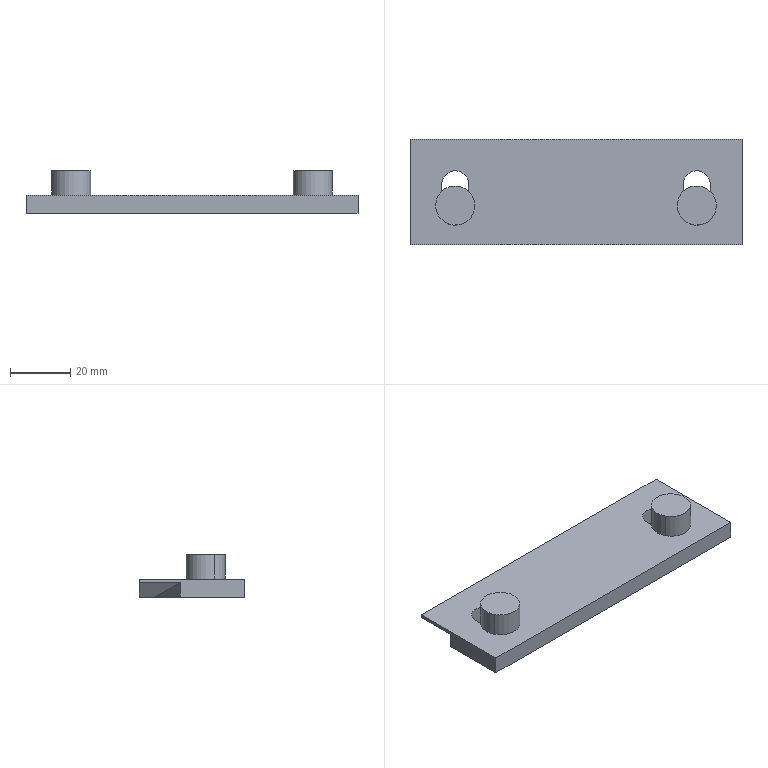Part | CATIA | 3 solids | 26 faces | box 110 x 35 x 14 mm | volume 22917 mm3 | plane 18 | cylinder 8 | commonest cylinder face diameters 9 x4 13 x4
STEP:
#1=CARTESIAN_POINT('',(-55.,-30.,38.));
#2=VERTEX_POINT('',#1);
#3=CARTESIAN_POINT('',(-55.,-30.,44.));
#4=VERTEX_POINT('',#3);
#5=CARTESIAN_POINT('',(-55.,-30.,41.));
#6=DIRECTION('',(0.,0.,1.));
#7=VECTOR('',#6,1.);
#8=LINE('',#5,#7);
#9=EDGE_CURVE('',#2,#4,#8,.T.);
#10=ORIENTED_EDGE('',*,*,#9,.F.);
#11=CARTESIAN_POINT('',(55.,-30.,38.));
#12=VERTEX_POINT('',#11);
#13=CARTESIAN_POINT('',(0.,-30.,38.));
#14=DIRECTION('',(1.,0.,0.));
#15=VECTOR('',#14,1.);
#16=LINE('',#13,#15);
#17=EDGE_CURVE('',#2,#12,#16,.T.);
#18=ORIENTED_EDGE('',*,*,#17,.T.);
#19=CARTESIAN_POINT('',(55.,-30.,44.));
#20=VERTEX_POINT('',#19);
#21=CARTESIAN_POINT('',(55.,-30.,41.));
#22=DIRECTION('',(0.,0.,1.));
#23=VECTOR('',#22,1.);
#24=LINE('',#21,#23);
#25=EDGE_CURVE('',#12,#20,#24,.T.);
#26=ORIENTED_EDGE('',*,*,#25,.T.);
#27=CARTESIAN_POINT('',(0.,-30.,44.));
#28=DIRECTION('',(1.,0.,0.));
#29=VECTOR('',#28,1.);
#30=LINE('',#27,#29);
#31=EDGE_CURVE('',#4,#20,#30,.T.);
#32=ORIENTED_EDGE('',*,*,#31,.F.);
#33=EDGE_LOOP('',(#10,#18,#26,#32));
#34=FACE_OUTER_BOUND('',#33,.T.);
#35=CARTESIAN_POINT('',(-55.,-30.,38.));
#36=DIRECTION('',(0.,-1.,0.));
#37=DIRECTION('',(1.,0.,0.));
#38=AXIS2_PLACEMENT_3D('',#35,#36,#37);
#39=PLANE('',#38);
#40=ADVANCED_FACE('',(#34),#39,.T.);
#41=CARTESIAN_POINT('',(55.,-8.66,42.874));
#42=VERTEX_POINT('',#41);
#43=CARTESIAN_POINT('',(55.,-8.66,38.));
#44=VERTEX_POINT('',#43);
#45=CARTESIAN_POINT('',(55.,-8.66,40.437));
#46=DIRECTION('',(0.,0.,-1.));
#47=VECTOR('',#46,1.);
#48=LINE('',#45,#47);
#49=EDGE_CURVE('',#42,#44,#48,.T.);
#50=ORIENTED_EDGE('',*,*,#49,.F.);
#51=CARTESIAN_POINT('',(55.,5.,42.874));
#52=VERTEX_POINT('',#51);
#53=CARTESIAN_POINT('',(55.,-1.83,42.874));
#54=DIRECTION('',(0.,1.,0.));
#55=VECTOR('',#54,1.);
#56=LINE('',#53,#55);
#57=EDGE_CURVE('',#42,#52,#56,.T.);
#58=ORIENTED_EDGE('',*,*,#57,.T.);
#59=CARTESIAN_POINT('',(55.,5.,44.));
#60=VERTEX_POINT('',#59);
#61=CARTESIAN_POINT('',(55.,5.,43.437));
#62=DIRECTION('',(0.,0.,1.));
#63=VECTOR('',#62,1.);
#64=LINE('',#61,#63);
#65=EDGE_CURVE('',#52,#60,#64,.T.);
#66=ORIENTED_EDGE('',*,*,#65,.T.);
#67=CARTESIAN_POINT('',(55.,-12.5,44.));
#68=DIRECTION('',(0.,-1.,0.));
#69=VECTOR('',#68,1.);
#70=LINE('',#67,#69);
#71=EDGE_CURVE('',#20,#60,#70,.F.);
#72=ORIENTED_EDGE('',*,*,#71,.F.);
#73=ORIENTED_EDGE('',*,*,#25,.F.);
#74=CARTESIAN_POINT('',(55.,-19.33,38.));
#75=DIRECTION('',(0.,-1.,0.));
#76=VECTOR('',#75,1.);
#77=LINE('',#74,#76);
#78=EDGE_CURVE('',#12,#44,#77,.F.);
#79=ORIENTED_EDGE('',*,*,#78,.T.);
#80=EDGE_LOOP('',(#50,#58,#66,#72,#73,#79));
#81=FACE_OUTER_BOUND('',#80,.T.);
#82=CARTESIAN_POINT('',(55.,5.,38.));
#83=DIRECTION('',(-1.,0.,0.));
#84=DIRECTION('',(0.,-1.,0.));
#85=AXIS2_PLACEMENT_3D('',#82,#83,#84);
#86=PLANE('',#85);
#87=ADVANCED_FACE('',(#81),#86,.F.);
#88=CARTESIAN_POINT('',(-55.,-8.66,42.874));
#89=VERTEX_POINT('',#88);
#90=CARTESIAN_POINT('',(-55.,5.,42.874));
#91=VERTEX_POINT('',#90);
#92=CARTESIAN_POINT('',(-55.,-1.83,42.874));
#93=DIRECTION('',(0.,1.,0.));
#94=VECTOR('',#93,1.);
#95=LINE('',#92,#94);
#96=EDGE_CURVE('',#89,#91,#95,.T.);
#97=ORIENTED_EDGE('',*,*,#96,.F.);
#98=CARTESIAN_POINT('',(-55.,-8.66,38.));
#99=VERTEX_POINT('',#98);
#100=CARTESIAN_POINT('',(-55.,-8.66,40.437));
#101=DIRECTION('',(0.,0.,-1.));
#102=VECTOR('',#101,1.);
#103=LINE('',#100,#102);
#104=EDGE_CURVE('',#89,#99,#103,.T.);
#105=ORIENTED_EDGE('',*,*,#104,.T.);
#106=CARTESIAN_POINT('',(-55.,-19.33,38.));
#107=DIRECTION('',(0.,1.,0.));
#108=VECTOR('',#107,1.);
#109=LINE('',#106,#108);
#110=EDGE_CURVE('',#99,#2,#109,.F.);
#111=ORIENTED_EDGE('',*,*,#110,.T.);
#112=ORIENTED_EDGE('',*,*,#9,.T.);
#113=CARTESIAN_POINT('',(-55.,5.,44.));
#114=VERTEX_POINT('',#113);
#115=CARTESIAN_POINT('',(-55.,-12.5,44.));
#116=DIRECTION('',(0.,1.,0.));
#117=VECTOR('',#116,1.);
#118=LINE('',#115,#117);
#119=EDGE_CURVE('',#114,#4,#118,.F.);
#120=ORIENTED_EDGE('',*,*,#119,.F.);
#121=CARTESIAN_POINT('',(-55.,5.,43.437));
#122=DIRECTION('',(0.,0.,1.));
#123=VECTOR('',#122,1.);
#124=LINE('',#121,#123);
#125=EDGE_CURVE('',#91,#114,#124,.T.);
#126=ORIENTED_EDGE('',*,*,#125,.F.);
#127=EDGE_LOOP('',(#97,#105,#111,#112,#120,#126));
#128=FACE_OUTER_BOUND('',#127,.T.);
#129=CARTESIAN_POINT('',(-55.,-30.,38.));
#130=DIRECTION('',(1.,0.,0.));
#131=DIRECTION('',(0.,1.,0.));
#132=AXIS2_PLACEMENT_3D('',#129,#130,#131);
#133=PLANE('',#132);
#134=ADVANCED_FACE('',(#128),#133,.F.);
#135=CARTESIAN_POINT('',(40.,5.,38.));
#136=VERTEX_POINT('',#135);
#137=CARTESIAN_POINT('',(-40.,5.,38.));
#138=VERTEX_POINT('',#137);
#139=CARTESIAN_POINT('',(0.,5.,38.));
#140=DIRECTION('',(-1.,0.,0.));
#141=VECTOR('',#140,1.);
#142=LINE('',#139,#141);
#143=EDGE_CURVE('',#136,#138,#142,.T.);
#144=ORIENTED_EDGE('',*,*,#143,.T.);
#145=CARTESIAN_POINT('',(-47.5,5.,40.437));
#146=DIRECTION('',(-0.9511,0.,0.309));
#147=VECTOR('',#146,1.);
#148=LINE('',#145,#147);
#149=EDGE_CURVE('',#138,#91,#148,.T.);
#150=ORIENTED_EDGE('',*,*,#149,.T.);
#151=ORIENTED_EDGE('',*,*,#125,.T.);
#152=CARTESIAN_POINT('',(0.,5.,44.));
#153=DIRECTION('',(-1.,0.,0.));
#154=VECTOR('',#153,1.);
#155=LINE('',#152,#154);
#156=EDGE_CURVE('',#60,#114,#155,.T.);
#157=ORIENTED_EDGE('',*,*,#156,.F.);
#158=ORIENTED_EDGE('',*,*,#65,.F.);
#159=CARTESIAN_POINT('',(47.5,5.,40.437));
#160=DIRECTION('',(0.9511,0.,0.309));
#161=VECTOR('',#160,1.);
#162=LINE('',#159,#161);
#163=EDGE_CURVE('',#136,#52,#162,.T.);
#164=ORIENTED_EDGE('',*,*,#163,.F.);
#165=EDGE_LOOP('',(#144,#150,#151,#157,#158,#164));
#166=FACE_OUTER_BOUND('',#165,.T.);
#167=CARTESIAN_POINT('',(55.,5.,38.));
#168=DIRECTION('',(0.,1.,0.));
#169=DIRECTION('',(-1.,0.,0.));
#170=AXIS2_PLACEMENT_3D('',#167,#168,#169);
#171=PLANE('',#170);
#172=ADVANCED_FACE('',(#166),#171,.T.);
#173=CARTESIAN_POINT('',(40.,0.,38.));
#174=VERTEX_POINT('',#173);
#175=CARTESIAN_POINT('',(55.,-8.66,42.874));
#176=CARTESIAN_POINT('',(40.,0.,38.));
#177=B_SPLINE_CURVE_WITH_KNOTS('',1,(#175,#176),.UNSPECIFIED.,.F.,.U.,(2,2),(-2.999,14.994),.UNSPECIFIED.);
#178=EDGE_CURVE('',#174,#42,#177,.F.);
#179=ORIENTED_EDGE('',*,*,#178,.T.);
#180=ORIENTED_EDGE('',*,*,#49,.T.);
#181=CARTESIAN_POINT('',(52.5,-7.217,38.));
#182=DIRECTION('',(0.866,-0.5,0.));
#183=VECTOR('',#182,1.);
#184=LINE('',#181,#183);
#185=EDGE_CURVE('',#174,#44,#184,.T.);
#186=ORIENTED_EDGE('',*,*,#185,.F.);
#187=EDGE_LOOP('',(#179,#180,#186));
#188=FACE_OUTER_BOUND('',#187,.T.);
#189=CARTESIAN_POINT('',(40.,0.,38.));
#190=DIRECTION('',(0.5,0.866,0.));
#191=DIRECTION('',(0.,0.,1.));
#192=AXIS2_PLACEMENT_3D('',#189,#190,#191);
#193=PLANE('',#192);
#194=ADVANCED_FACE('',(#188),#193,.T.);
#195=ORIENTED_EDGE('',*,*,#163,.T.);
#196=ORIENTED_EDGE('',*,*,#57,.F.);
#197=ORIENTED_EDGE('',*,*,#178,.F.);
#198=CARTESIAN_POINT('',(40.,5.,38.));
#199=DIRECTION('',(0.,-1.,0.));
#200=VECTOR('',#199,1.);
#201=LINE('',#198,#200);
#202=EDGE_CURVE('',#174,#136,#201,.F.);
#203=ORIENTED_EDGE('',*,*,#202,.T.);
#204=EDGE_LOOP('',(#195,#196,#197,#203));
#205=FACE_OUTER_BOUND('',#204,.T.);
#206=CARTESIAN_POINT('',(40.,10.,38.));
#207=DIRECTION('',(-0.309,0.,0.9511));
#208=DIRECTION('',(0.,-1.,0.));
#209=AXIS2_PLACEMENT_3D('',#206,#207,#208);
#210=PLANE('',#209);
#211=ADVANCED_FACE('',(#205),#210,.F.);
#212=CARTESIAN_POINT('',(-40.,0.,38.));
#213=VERTEX_POINT('',#212);
#214=CARTESIAN_POINT('',(-52.5,-7.217,38.));
#215=DIRECTION('',(-0.866,-0.5,0.));
#216=VECTOR('',#215,1.);
#217=LINE('',#214,#216);
#218=EDGE_CURVE('',#213,#99,#217,.T.);
#219=ORIENTED_EDGE('',*,*,#218,.T.);
#220=ORIENTED_EDGE('',*,*,#104,.F.);
#221=CARTESIAN_POINT('',(-55.,-8.66,42.874));
#222=CARTESIAN_POINT('',(-40.,0.,38.));
#223=B_SPLINE_CURVE_WITH_KNOTS('',1,(#221,#222),.UNSPECIFIED.,.F.,.U.,(2,2),(-2.999,14.994),.UNSPECIFIED.);
#224=EDGE_CURVE('',#213,#89,#223,.F.);
#225=ORIENTED_EDGE('',*,*,#224,.F.);
#226=EDGE_LOOP('',(#219,#220,#225));
#227=FACE_OUTER_BOUND('',#226,.T.);
#228=CARTESIAN_POINT('',(-40.,0.,38.));
#229=DIRECTION('',(0.5,-0.866,0.));
#230=DIRECTION('',(0.,0.,1.));
#231=AXIS2_PLACEMENT_3D('',#228,#229,#230);
#232=PLANE('',#231);
#233=ADVANCED_FACE('',(#227),#232,.F.);
#234=CARTESIAN_POINT('',(-40.,5.,38.));
#235=DIRECTION('',(0.,-1.,0.));
#236=VECTOR('',#235,1.);
#237=LINE('',#234,#236);
#238=EDGE_CURVE('',#213,#138,#237,.F.);
#239=ORIENTED_EDGE('',*,*,#238,.F.);
#240=ORIENTED_EDGE('',*,*,#224,.T.);
#241=ORIENTED_EDGE('',*,*,#96,.T.);
#242=ORIENTED_EDGE('',*,*,#149,.F.);
#243=EDGE_LOOP('',(#239,#240,#241,#242));
#244=FACE_OUTER_BOUND('',#243,.T.);
#245=CARTESIAN_POINT('',(-40.,10.,38.));
#246=DIRECTION('',(-0.309,0.,-0.9511));
#247=DIRECTION('',(0.,-1.,0.));
#248=AXIS2_PLACEMENT_3D('',#245,#246,#247);
#249=PLANE('',#248);
#250=ADVANCED_FACE('',(#244),#249,.T.);
#251=ORIENTED_EDGE('',*,*,#143,.F.);
#252=ORIENTED_EDGE('',*,*,#202,.F.);
#253=ORIENTED_EDGE('',*,*,#185,.T.);
#254=ORIENTED_EDGE('',*,*,#78,.F.);
#255=ORIENTED_EDGE('',*,*,#17,.F.);
#256=ORIENTED_EDGE('',*,*,#110,.F.);
#257=ORIENTED_EDGE('',*,*,#218,.F.);
#258=ORIENTED_EDGE('',*,*,#238,.T.);
#259=EDGE_LOOP('',(#251,#252,#253,#254,#255,#256,#257,#258));
#260=FACE_OUTER_BOUND('',#259,.T.);
#261=CARTESIAN_POINT('',(-35.5,-10.,38.));
#262=VERTEX_POINT('',#261);
#263=CARTESIAN_POINT('',(-35.5,-17.,38.));
#264=VERTEX_POINT('',#263);
#265=CARTESIAN_POINT('',(-35.5,-13.5,38.));
#266=DIRECTION('',(0.,-1.,0.));
#267=VECTOR('',#266,1.);
#268=LINE('',#265,#267);
#269=EDGE_CURVE('',#262,#264,#268,.T.);
#270=ORIENTED_EDGE('',*,*,#269,.F.);
#271=CARTESIAN_POINT('',(-44.5,-10.,38.));
#272=VERTEX_POINT('',#271);
#273=CARTESIAN_POINT('',(-40.,-10.,38.));
#274=DIRECTION('',(0.,0.,1.));
#275=AXIS2_PLACEMENT_3D('',#273,#274,$);
#276=CIRCLE('',#275,4.5);
#277=EDGE_CURVE('',#262,#272,#276,.T.);
#278=ORIENTED_EDGE('',*,*,#277,.T.);
#279=CARTESIAN_POINT('',(-44.5,-17.,38.));
#280=VERTEX_POINT('',#279);
#281=CARTESIAN_POINT('',(-44.5,-13.5,38.));
#282=DIRECTION('',(0.,-1.,0.));
#283=VECTOR('',#282,1.);
#284=LINE('',#281,#283);
#285=EDGE_CURVE('',#272,#280,#284,.T.);
#286=ORIENTED_EDGE('',*,*,#285,.T.);
#287=CARTESIAN_POINT('',(-40.,-17.,38.));
#288=DIRECTION('',(0.,0.,1.));
#289=AXIS2_PLACEMENT_3D('',#287,#288,$);
#290=CIRCLE('',#289,4.5);
#291=EDGE_CURVE('',#280,#264,#290,.T.);
#292=ORIENTED_EDGE('',*,*,#291,.T.);
#293=EDGE_LOOP('',(#270,#278,#286,#292));
#294=FACE_BOUND('',#293,.T.);
#295=CARTESIAN_POINT('',(44.5,-10.,38.));
#296=VERTEX_POINT('',#295);
#297=CARTESIAN_POINT('',(35.5,-10.,38.));
#298=VERTEX_POINT('',#297);
#299=CARTESIAN_POINT('',(40.,-10.,38.));
#300=DIRECTION('',(0.,0.,1.));
#301=AXIS2_PLACEMENT_3D('',#299,#300,$);
#302=CIRCLE('',#301,4.5);
#303=EDGE_CURVE('',#296,#298,#302,.T.);
#304=ORIENTED_EDGE('',*,*,#303,.T.);
#305=CARTESIAN_POINT('',(35.5,-17.,38.));
#306=VERTEX_POINT('',#305);
#307=CARTESIAN_POINT('',(35.5,-13.5,38.));
#308=DIRECTION('',(0.,-1.,0.));
#309=VECTOR('',#308,1.);
#310=LINE('',#307,#309);
#311=EDGE_CURVE('',#298,#306,#310,.T.);
#312=ORIENTED_EDGE('',*,*,#311,.T.);
#313=CARTESIAN_POINT('',(44.5,-17.,38.));
#314=VERTEX_POINT('',#313);
#315=CARTESIAN_POINT('',(40.,-17.,38.));
#316=DIRECTION('',(0.,0.,1.));
#317=AXIS2_PLACEMENT_3D('',#315,#316,$);
#318=CIRCLE('',#317,4.5);
#319=EDGE_CURVE('',#306,#314,#318,.T.);
#320=ORIENTED_EDGE('',*,*,#319,.T.);
#321=CARTESIAN_POINT('',(44.5,-13.5,38.));
#322=DIRECTION('',(0.,-1.,0.));
#323=VECTOR('',#322,1.);
#324=LINE('',#321,#323);
#325=EDGE_CURVE('',#296,#314,#324,.T.);
#326=ORIENTED_EDGE('',*,*,#325,.F.);
#327=EDGE_LOOP('',(#304,#312,#320,#326));
#328=FACE_BOUND('',#327,.T.);
#329=CARTESIAN_POINT('',(0.,0.,38.));
#330=DIRECTION('',(0.,0.,1.));
#331=DIRECTION('',(1.,0.,0.));
#332=AXIS2_PLACEMENT_3D('',#329,#330,#331);
#333=PLANE('',#332);
#334=ADVANCED_FACE('',(#260,#294,#328),#333,.F.);
#335=ORIENTED_EDGE('',*,*,#156,.T.);
#336=ORIENTED_EDGE('',*,*,#119,.T.);
#337=ORIENTED_EDGE('',*,*,#31,.T.);
#338=ORIENTED_EDGE('',*,*,#71,.T.);
#339=EDGE_LOOP('',(#335,#336,#337,#338));
#340=FACE_OUTER_BOUND('',#339,.T.);
#341=CARTESIAN_POINT('',(-35.5,-17.,44.));
#342=VERTEX_POINT('',#341);
#343=CARTESIAN_POINT('',(-35.5,-10.,44.));
#344=VERTEX_POINT('',#343);
#345=CARTESIAN_POINT('',(-35.5,-13.5,44.));
#346=DIRECTION('',(0.,-1.,0.));
#347=VECTOR('',#346,1.);
#348=LINE('',#345,#347);
#349=EDGE_CURVE('',#342,#344,#348,.F.);
#350=ORIENTED_EDGE('',*,*,#349,.F.);
#351=CARTESIAN_POINT('',(-44.5,-17.,44.));
#352=VERTEX_POINT('',#351);
#353=CARTESIAN_POINT('',(-40.,-17.,44.));
#354=DIRECTION('',(0.,0.,1.));
#355=AXIS2_PLACEMENT_3D('',#353,#354,$);
#356=CIRCLE('',#355,4.5);
#357=EDGE_CURVE('',#352,#342,#356,.T.);
#358=ORIENTED_EDGE('',*,*,#357,.F.);
#359=CARTESIAN_POINT('',(-44.5,-10.,44.));
#360=VERTEX_POINT('',#359);
#361=CARTESIAN_POINT('',(-44.5,-13.5,44.));
#362=DIRECTION('',(0.,-1.,0.));
#363=VECTOR('',#362,1.);
#364=LINE('',#361,#363);
#365=EDGE_CURVE('',#360,#352,#364,.T.);
#366=ORIENTED_EDGE('',*,*,#365,.F.);
#367=CARTESIAN_POINT('',(-40.,-10.,44.));
#368=DIRECTION('',(0.,0.,1.));
#369=AXIS2_PLACEMENT_3D('',#367,#368,$);
#370=CIRCLE('',#369,4.5);
#371=EDGE_CURVE('',#344,#360,#370,.T.);
#372=ORIENTED_EDGE('',*,*,#371,.F.);
#373=EDGE_LOOP('',(#350,#358,#366,#372));
#374=FACE_BOUND('',#373,.T.);
#375=CARTESIAN_POINT('',(44.5,-10.,44.));
#376=VERTEX_POINT('',#375);
#377=CARTESIAN_POINT('',(35.5,-10.,44.));
#378=VERTEX_POINT('',#377);
#379=CARTESIAN_POINT('',(40.,-10.,44.));
#380=DIRECTION('',(0.,0.,1.));
#381=AXIS2_PLACEMENT_3D('',#379,#380,$);
#382=CIRCLE('',#381,4.5);
#383=EDGE_CURVE('',#376,#378,#382,.T.);
#384=ORIENTED_EDGE('',*,*,#383,.F.);
#385=CARTESIAN_POINT('',(44.5,-17.,44.));
#386=VERTEX_POINT('',#385);
#387=CARTESIAN_POINT('',(44.5,-13.5,44.));
#388=DIRECTION('',(0.,-1.,0.));
#389=VECTOR('',#388,1.);
#390=LINE('',#387,#389);
#391=EDGE_CURVE('',#386,#376,#390,.F.);
#392=ORIENTED_EDGE('',*,*,#391,.F.);
#393=CARTESIAN_POINT('',(35.5,-17.,44.));
#394=VERTEX_POINT('',#393);
#395=CARTESIAN_POINT('',(40.,-17.,44.));
#396=DIRECTION('',(0.,0.,1.));
#397=AXIS2_PLACEMENT_3D('',#395,#396,$);
#398=CIRCLE('',#397,4.5);
#399=EDGE_CURVE('',#394,#386,#398,.T.);
#400=ORIENTED_EDGE('',*,*,#399,.F.);
#401=CARTESIAN_POINT('',(35.5,-13.5,44.));
#402=DIRECTION('',(0.,-1.,0.));
#403=VECTOR('',#402,1.);
#404=LINE('',#401,#403);
#405=EDGE_CURVE('',#378,#394,#404,.T.);
#406=ORIENTED_EDGE('',*,*,#405,.F.);
#407=EDGE_LOOP('',(#384,#392,#400,#406));
#408=FACE_BOUND('',#407,.T.);
#409=CARTESIAN_POINT('',(0.,0.,44.));
#410=DIRECTION('',(0.,0.,1.));
#411=DIRECTION('',(1.,0.,0.));
#412=AXIS2_PLACEMENT_3D('',#409,#410,#411);
#413=PLANE('',#412);
#414=ADVANCED_FACE('',(#340,#374,#408),#413,.T.);
#415=ORIENTED_EDGE('',*,*,#303,.F.);
#416=CARTESIAN_POINT('',(44.5,-10.,34.));
#417=DIRECTION('',(0.,0.,1.));
#418=VECTOR('',#417,1.);
#419=LINE('',#416,#418);
#420=EDGE_CURVE('',#376,#296,#419,.F.);
#421=ORIENTED_EDGE('',*,*,#420,.F.);
#422=ORIENTED_EDGE('',*,*,#383,.T.);
#423=CARTESIAN_POINT('',(35.5,-10.,34.));
#424=DIRECTION('',(0.,0.,1.));
#425=VECTOR('',#424,1.);
#426=LINE('',#423,#425);
#427=EDGE_CURVE('',#378,#298,#426,.F.);
#428=ORIENTED_EDGE('',*,*,#427,.T.);
#429=EDGE_LOOP('',(#415,#421,#422,#428));
#430=FACE_OUTER_BOUND('',#429,.T.);
#431=CARTESIAN_POINT('',(40.,-10.,34.));
#432=DIRECTION('',(0.,0.,1.));
#433=DIRECTION('',(1.,0.,0.));
#434=AXIS2_PLACEMENT_3D('',#431,#432,#433);
#435=CYLINDRICAL_SURFACE('',#434,4.5);
#436=ADVANCED_FACE('',(#430),#435,.F.);
#437=ORIENTED_EDGE('',*,*,#427,.F.);
#438=ORIENTED_EDGE('',*,*,#405,.T.);
#439=CARTESIAN_POINT('',(35.5,-17.,41.));
#440=DIRECTION('',(0.,0.,-1.));
#441=VECTOR('',#440,1.);
#442=LINE('',#439,#441);
#443=EDGE_CURVE('',#394,#306,#442,.T.);
#444=ORIENTED_EDGE('',*,*,#443,.T.);
#445=ORIENTED_EDGE('',*,*,#311,.F.);
#446=EDGE_LOOP('',(#437,#438,#444,#445));
#447=FACE_OUTER_BOUND('',#446,.T.);
#448=CARTESIAN_POINT('',(35.5,-10.,44.));
#449=DIRECTION('',(1.,0.,0.));
#450=DIRECTION('',(0.,-1.,0.));
#451=AXIS2_PLACEMENT_3D('',#448,#449,#450);
#452=PLANE('',#451);
#453=ADVANCED_FACE('',(#447),#452,.T.);
#454=ORIENTED_EDGE('',*,*,#325,.T.);
#455=CARTESIAN_POINT('',(44.5,-17.,41.));
#456=DIRECTION('',(0.,0.,-1.));
#457=VECTOR('',#456,1.);
#458=LINE('',#455,#457);
#459=EDGE_CURVE('',#386,#314,#458,.T.);
#460=ORIENTED_EDGE('',*,*,#459,.F.);
#461=ORIENTED_EDGE('',*,*,#391,.T.);
#462=ORIENTED_EDGE('',*,*,#420,.T.);
#463=EDGE_LOOP('',(#454,#460,#461,#462));
#464=FACE_OUTER_BOUND('',#463,.T.);
#465=CARTESIAN_POINT('',(44.5,-10.,44.));
#466=DIRECTION('',(1.,0.,0.));
#467=DIRECTION('',(0.,-1.,0.));
#468=AXIS2_PLACEMENT_3D('',#465,#466,#467);
#469=PLANE('',#468);
#470=ADVANCED_FACE('',(#464),#469,.F.);
#471=ORIENTED_EDGE('',*,*,#319,.F.);
#472=ORIENTED_EDGE('',*,*,#443,.F.);
#473=ORIENTED_EDGE('',*,*,#399,.T.);
#474=ORIENTED_EDGE('',*,*,#459,.T.);
#475=EDGE_LOOP('',(#471,#472,#473,#474));
#476=FACE_OUTER_BOUND('',#475,.T.);
#477=CARTESIAN_POINT('',(40.,-17.,34.));
#478=DIRECTION('',(0.,0.,1.));
#479=DIRECTION('',(-1.,0.,0.));
#480=AXIS2_PLACEMENT_3D('',#477,#478,#479);
#481=CYLINDRICAL_SURFACE('',#480,4.5);
#482=ADVANCED_FACE('',(#476),#481,.F.);
#483=ORIENTED_EDGE('',*,*,#269,.T.);
#484=CARTESIAN_POINT('',(-35.5,-17.,41.));
#485=DIRECTION('',(0.,0.,-1.));
#486=VECTOR('',#485,1.);
#487=LINE('',#484,#486);
#488=EDGE_CURVE('',#342,#264,#487,.T.);
#489=ORIENTED_EDGE('',*,*,#488,.F.);
#490=ORIENTED_EDGE('',*,*,#349,.T.);
#491=CARTESIAN_POINT('',(-35.5,-10.,41.));
#492=DIRECTION('',(0.,0.,-1.));
#493=VECTOR('',#492,1.);
#494=LINE('',#491,#493);
#495=EDGE_CURVE('',#344,#262,#494,.T.);
#496=ORIENTED_EDGE('',*,*,#495,.T.);
#497=EDGE_LOOP('',(#483,#489,#490,#496));
#498=FACE_OUTER_BOUND('',#497,.T.);
#499=CARTESIAN_POINT('',(-35.5,-10.,44.));
#500=DIRECTION('',(1.,0.,0.));
#501=DIRECTION('',(0.,-1.,0.));
#502=AXIS2_PLACEMENT_3D('',#499,#500,#501);
#503=PLANE('',#502);
#504=ADVANCED_FACE('',(#498),#503,.F.);
#505=ORIENTED_EDGE('',*,*,#277,.F.);
#506=ORIENTED_EDGE('',*,*,#495,.F.);
#507=ORIENTED_EDGE('',*,*,#371,.T.);
#508=CARTESIAN_POINT('',(-44.5,-10.,34.));
#509=DIRECTION('',(0.,0.,1.));
#510=VECTOR('',#509,1.);
#511=LINE('',#508,#510);
#512=EDGE_CURVE('',#360,#272,#511,.F.);
#513=ORIENTED_EDGE('',*,*,#512,.T.);
#514=EDGE_LOOP('',(#505,#506,#507,#513));
#515=FACE_OUTER_BOUND('',#514,.T.);
#516=CARTESIAN_POINT('',(-40.,-10.,34.));
#517=DIRECTION('',(0.,0.,1.));
#518=DIRECTION('',(1.,0.,0.));
#519=AXIS2_PLACEMENT_3D('',#516,#517,#518);
#520=CYLINDRICAL_SURFACE('',#519,4.5);
#521=ADVANCED_FACE('',(#515),#520,.F.);
#522=ORIENTED_EDGE('',*,*,#291,.F.);
#523=CARTESIAN_POINT('',(-44.5,-17.,34.));
#524=DIRECTION('',(0.,0.,1.));
#525=VECTOR('',#524,1.);
#526=LINE('',#523,#525);
#527=EDGE_CURVE('',#352,#280,#526,.F.);
#528=ORIENTED_EDGE('',*,*,#527,.F.);
#529=ORIENTED_EDGE('',*,*,#357,.T.);
#530=ORIENTED_EDGE('',*,*,#488,.T.);
#531=EDGE_LOOP('',(#522,#528,#529,#530));
#532=FACE_OUTER_BOUND('',#531,.T.);
#533=CARTESIAN_POINT('',(-40.,-17.,34.));
#534=DIRECTION('',(0.,0.,1.));
#535=DIRECTION('',(-1.,0.,0.));
#536=AXIS2_PLACEMENT_3D('',#533,#534,#535);
#537=CYLINDRICAL_SURFACE('',#536,4.5);
#538=ADVANCED_FACE('',(#532),#537,.F.);
#539=ORIENTED_EDGE('',*,*,#512,.F.);
#540=ORIENTED_EDGE('',*,*,#365,.T.);
#541=ORIENTED_EDGE('',*,*,#527,.T.);
#542=ORIENTED_EDGE('',*,*,#285,.F.);
#543=EDGE_LOOP('',(#539,#540,#541,#542));
#544=FACE_OUTER_BOUND('',#543,.T.);
#545=CARTESIAN_POINT('',(-44.5,-10.,44.));
#546=DIRECTION('',(1.,0.,0.));
#547=DIRECTION('',(0.,-1.,0.));
#548=AXIS2_PLACEMENT_3D('',#545,#546,#547);
#549=PLANE('',#548);
#550=ADVANCED_FACE('',(#544),#549,.T.);
#551=CLOSED_SHELL('',(#40,#87,#134,#172,#194,#211,#233,#250,#334,#414,#436,#453,#470,#482,#504,#521,#538,#550));
#552=MANIFOLD_SOLID_BREP('',#551);
#553=CARTESIAN_POINT('',(-34.296,-13.884,52.));
#554=VERTEX_POINT('',#553);
#555=CARTESIAN_POINT('',(-45.704,-20.116,52.));
#556=VERTEX_POINT('',#555);
#557=CARTESIAN_POINT('',(-40.,-17.,52.));
#558=DIRECTION('',(0.,0.,1.));
#559=AXIS2_PLACEMENT_3D('',#557,#558,$);
#560=CIRCLE('',#559,6.5);
#561=EDGE_CURVE('',#554,#556,#560,.T.);
#562=ORIENTED_EDGE('',*,*,#561,.T.);
#563=CARTESIAN_POINT('',(-40.,-17.,52.));
#564=DIRECTION('',(0.,0.,1.));
#565=AXIS2_PLACEMENT_3D('',#563,#564,$);
#566=CIRCLE('',#565,6.5);
#567=EDGE_CURVE('',#556,#554,#566,.T.);
#568=ORIENTED_EDGE('',*,*,#567,.T.);
#569=EDGE_LOOP('',(#562,#568));
#570=FACE_OUTER_BOUND('',#569,.T.);
#571=CARTESIAN_POINT('',(-40.,-17.,52.));
#572=DIRECTION('',(0.,0.,1.));
#573=DIRECTION('',(1.,0.,0.));
#574=AXIS2_PLACEMENT_3D('',#571,#572,#573);
#575=PLANE('',#574);
#576=ADVANCED_FACE('',(#570),#575,.T.);
#577=CARTESIAN_POINT('',(-45.704,-20.116,44.));
#578=VERTEX_POINT('',#577);
#579=CARTESIAN_POINT('',(-45.704,-20.116,47.8));
#580=DIRECTION('',(0.,0.,1.));
#581=VECTOR('',#580,1.);
#582=LINE('',#579,#581);
#583=EDGE_CURVE('',#556,#578,#582,.F.);
#584=ORIENTED_EDGE('',*,*,#583,.F.);
#585=ORIENTED_EDGE('',*,*,#561,.F.);
#586=CARTESIAN_POINT('',(-34.296,-13.884,44.));
#587=VERTEX_POINT('',#586);
#588=CARTESIAN_POINT('',(-34.296,-13.884,47.8));
#589=DIRECTION('',(0.,0.,1.));
#590=VECTOR('',#589,1.);
#591=LINE('',#588,#590);
#592=EDGE_CURVE('',#554,#587,#591,.F.);
#593=ORIENTED_EDGE('',*,*,#592,.T.);
#594=CARTESIAN_POINT('',(-40.,-17.,44.));
#595=DIRECTION('',(0.,0.,1.));
#596=AXIS2_PLACEMENT_3D('',#594,#595,$);
#597=CIRCLE('',#596,6.5);
#598=EDGE_CURVE('',#587,#578,#597,.T.);
#599=ORIENTED_EDGE('',*,*,#598,.T.);
#600=EDGE_LOOP('',(#584,#585,#593,#599));
#601=FACE_OUTER_BOUND('',#600,.T.);
#602=CARTESIAN_POINT('',(-40.,-17.,44.1));
#603=DIRECTION('',(0.,0.,1.));
#604=DIRECTION('',(0.8776,0.4794,0.));
#605=AXIS2_PLACEMENT_3D('',#602,#603,#604);
#606=CYLINDRICAL_SURFACE('',#605,6.5);
#607=ADVANCED_FACE('',(#601),#606,.T.);
#608=ORIENTED_EDGE('',*,*,#592,.F.);
#609=ORIENTED_EDGE('',*,*,#567,.F.);
#610=ORIENTED_EDGE('',*,*,#583,.T.);
#611=CARTESIAN_POINT('',(-40.,-17.,44.));
#612=DIRECTION('',(0.,0.,1.));
#613=AXIS2_PLACEMENT_3D('',#611,#612,$);
#614=CIRCLE('',#613,6.5);
#615=EDGE_CURVE('',#578,#587,#614,.T.);
#616=ORIENTED_EDGE('',*,*,#615,.T.);
#617=EDGE_LOOP('',(#608,#609,#610,#616));
#618=FACE_OUTER_BOUND('',#617,.T.);
#619=ADVANCED_FACE('',(#618),#606,.T.);
#620=ORIENTED_EDGE('',*,*,#598,.F.);
#621=ORIENTED_EDGE('',*,*,#615,.F.);
#622=EDGE_LOOP('',(#620,#621));
#623=FACE_OUTER_BOUND('',#622,.T.);
#624=ADVANCED_FACE('',(#623),#413,.F.);
#625=CLOSED_SHELL('',(#576,#607,#619,#624));
#626=MANIFOLD_SOLID_BREP('',#625);
#627=CARTESIAN_POINT('',(45.704,-13.884,52.));
#628=VERTEX_POINT('',#627);
#629=CARTESIAN_POINT('',(34.296,-20.116,52.));
#630=VERTEX_POINT('',#629);
#631=CARTESIAN_POINT('',(40.,-17.,52.));
#632=DIRECTION('',(0.,0.,1.));
#633=AXIS2_PLACEMENT_3D('',#631,#632,$);
#634=CIRCLE('',#633,6.5);
#635=EDGE_CURVE('',#628,#630,#634,.T.);
#636=ORIENTED_EDGE('',*,*,#635,.T.);
#637=CARTESIAN_POINT('',(40.,-17.,52.));
#638=DIRECTION('',(0.,0.,1.));
#639=AXIS2_PLACEMENT_3D('',#637,#638,$);
#640=CIRCLE('',#639,6.5);
#641=EDGE_CURVE('',#630,#628,#640,.T.);
#642=ORIENTED_EDGE('',*,*,#641,.T.);
#643=EDGE_LOOP('',(#636,#642));
#644=FACE_OUTER_BOUND('',#643,.T.);
#645=ADVANCED_FACE('',(#644),#575,.T.);
#646=CARTESIAN_POINT('',(34.296,-20.116,44.));
#647=VERTEX_POINT('',#646);
#648=CARTESIAN_POINT('',(34.296,-20.116,47.8));
#649=DIRECTION('',(0.,0.,1.));
#650=VECTOR('',#649,1.);
#651=LINE('',#648,#650);
#652=EDGE_CURVE('',#630,#647,#651,.F.);
#653=ORIENTED_EDGE('',*,*,#652,.F.);
#654=ORIENTED_EDGE('',*,*,#635,.F.);
#655=CARTESIAN_POINT('',(45.704,-13.884,44.));
#656=VERTEX_POINT('',#655);
#657=CARTESIAN_POINT('',(45.704,-13.884,47.8));
#658=DIRECTION('',(0.,0.,1.));
#659=VECTOR('',#658,1.);
#660=LINE('',#657,#659);
#661=EDGE_CURVE('',#628,#656,#660,.F.);
#662=ORIENTED_EDGE('',*,*,#661,.T.);
#663=CARTESIAN_POINT('',(40.,-17.,44.));
#664=DIRECTION('',(0.,0.,1.));
#665=AXIS2_PLACEMENT_3D('',#663,#664,$);
#666=CIRCLE('',#665,6.5);
#667=EDGE_CURVE('',#656,#647,#666,.T.);
#668=ORIENTED_EDGE('',*,*,#667,.T.);
#669=EDGE_LOOP('',(#653,#654,#662,#668));
#670=FACE_OUTER_BOUND('',#669,.T.);
#671=CARTESIAN_POINT('',(40.,-17.,44.1));
#672=DIRECTION('',(0.,0.,1.));
#673=DIRECTION('',(0.8776,0.4794,0.));
#674=AXIS2_PLACEMENT_3D('',#671,#672,#673);
#675=CYLINDRICAL_SURFACE('',#674,6.5);
#676=ADVANCED_FACE('',(#670),#675,.T.);
#677=ORIENTED_EDGE('',*,*,#661,.F.);
#678=ORIENTED_EDGE('',*,*,#641,.F.);
#679=ORIENTED_EDGE('',*,*,#652,.T.);
#680=CARTESIAN_POINT('',(40.,-17.,44.));
#681=DIRECTION('',(0.,0.,1.));
#682=AXIS2_PLACEMENT_3D('',#680,#681,$);
#683=CIRCLE('',#682,6.5);
#684=EDGE_CURVE('',#647,#656,#683,.T.);
#685=ORIENTED_EDGE('',*,*,#684,.T.);
#686=EDGE_LOOP('',(#677,#678,#679,#685));
#687=FACE_OUTER_BOUND('',#686,.T.);
#688=ADVANCED_FACE('',(#687),#675,.T.);
#689=ORIENTED_EDGE('',*,*,#667,.F.);
#690=ORIENTED_EDGE('',*,*,#684,.F.);
#691=EDGE_LOOP('',(#689,#690));
#692=FACE_OUTER_BOUND('',#691,.T.);
#693=ADVANCED_FACE('',(#692),#413,.F.);
#694=CLOSED_SHELL('',(#645,#676,#688,#693));
#695=MANIFOLD_SOLID_BREP('',#694);
#696=(LENGTH_UNIT()NAMED_UNIT(*)SI_UNIT(.MILLI.,.METRE.));
#697=UNCERTAINTY_MEASURE_WITH_UNIT(LENGTH_MEASURE(0.005),#696,'','');
#698=(NAMED_UNIT(*)PLANE_ANGLE_UNIT()SI_UNIT($,.RADIAN.));
#699=(NAMED_UNIT(*)SI_UNIT($,.STERADIAN.)SOLID_ANGLE_UNIT());
#700=(GEOMETRIC_REPRESENTATION_CONTEXT(3)GLOBAL_UNCERTAINTY_ASSIGNED_CONTEXT((#697))GLOBAL_UNIT_ASSIGNED_CONTEXT((#696,#698,#699))REPRESENTATION_CONTEXT('',''));
#701=ADVANCED_BREP_SHAPE_REPRESENTATION('',(#552,#626,#695),#700);